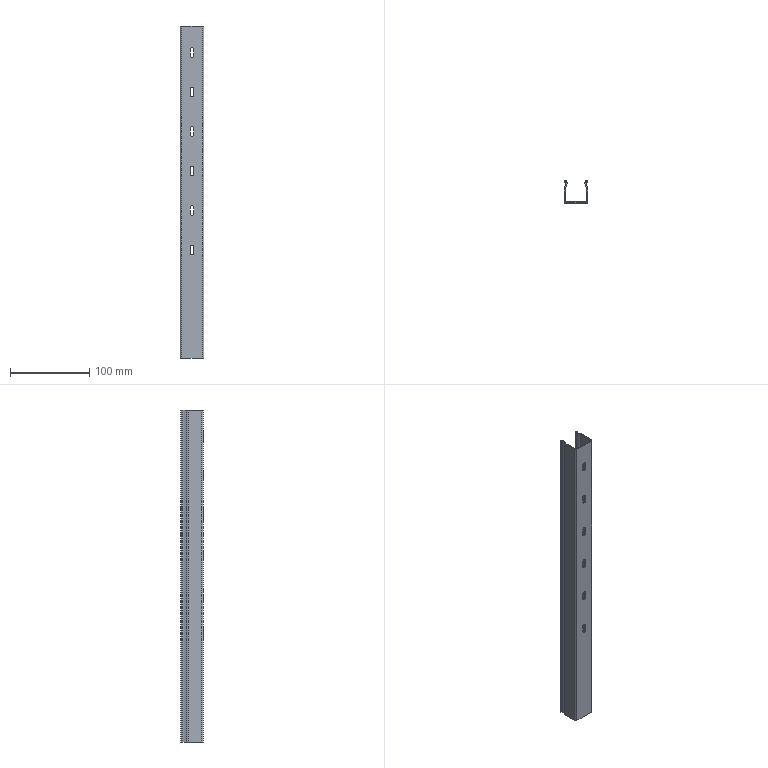Part | SolidWorks | features BaseBody 1 | 1 solid | 62 faces | box 30 x 28 x 420 mm | volume 45183 mm3 | cylinder 36 | plane 26 | commonest cylinder face diameters 5 x18 2 x3 4.5 x3 1.5 x2 3.5 x2 4 x2